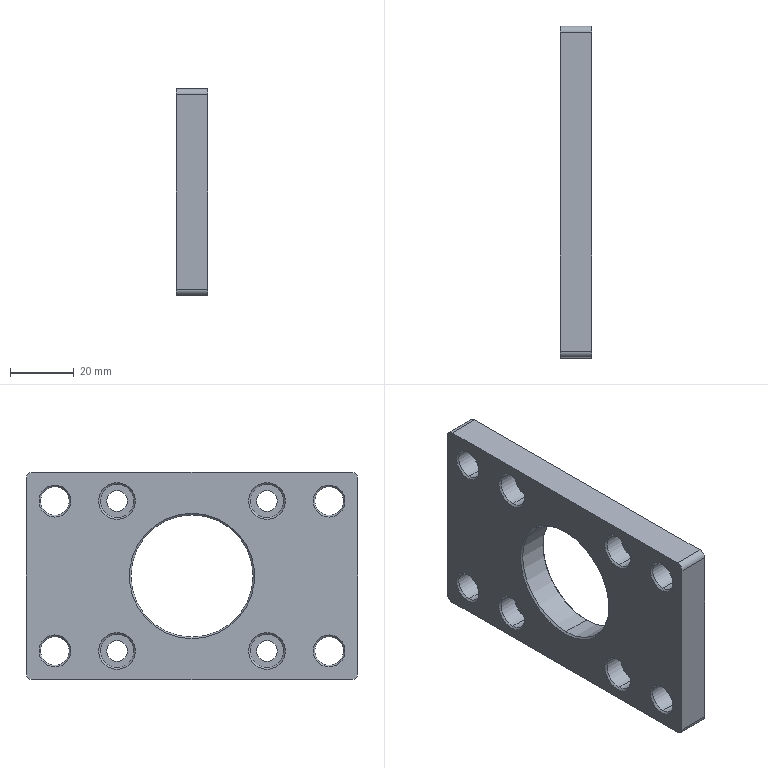Part | SolidWorks | features RefAxis 15, 3DProfileFeature 5, RevCut 3, LPattern 2, Extrusion 1 | 1 solid | 60 faces | box 10 x 104 x 65 mm | volume 50722 mm3 | cylinder 30 | cone 20 | plane 10 | commonest cylinder face diameters 6.5 x8 9 x8 10.5 x8 4 x4 38.3 x2